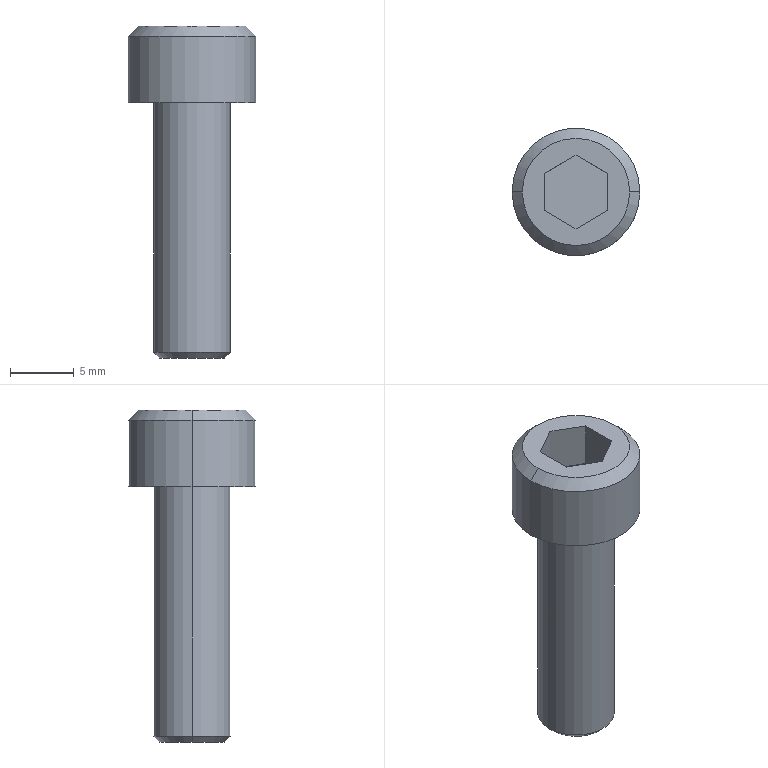Part | Creo | 1 solid | 18 faces | box 10 x 10 x 26 mm | volume 947.453 mm3 | plane 10 | cylinder 4 | cone 4 | commonest cylinder face diameters 6 x2 10 x2
STEP:
#1=CARTESIAN_POINT('',(-109.033,-193.,47.5));
#2=VERTEX_POINT('',#1);
#3=CARTESIAN_POINT('',(-119.033,-193.,47.5));
#4=VERTEX_POINT('',#3);
#5=CARTESIAN_POINT('',(-114.033,-193.,47.5));
#6=DIRECTION('',(0.,0.,-1.));
#7=DIRECTION('',(1.,0.,0.));
#8=AXIS2_PLACEMENT_3D('',#5,#6,#7);
#9=CIRCLE('',#8,5.);
#10=EDGE_CURVE('',#2,#4,#9,.T.);
#11=ORIENTED_EDGE('',*,*,#10,.F.);
#12=CARTESIAN_POINT('',(-114.033,-193.,47.5));
#13=DIRECTION('',(0.,0.,-1.));
#14=DIRECTION('',(-1.,0.,0.));
#15=AXIS2_PLACEMENT_3D('',#12,#13,#14);
#16=CIRCLE('',#15,5.);
#17=EDGE_CURVE('',#4,#2,#16,.T.);
#18=ORIENTED_EDGE('',*,*,#17,.F.);
#19=EDGE_LOOP('',(#11,#18));
#20=FACE_OUTER_BOUND('',#19,.F.);
#21=CARTESIAN_POINT('',(-117.033,-193.,47.5));
#22=VERTEX_POINT('',#21);
#23=CARTESIAN_POINT('',(-111.033,-193.,47.5));
#24=VERTEX_POINT('',#23);
#25=CARTESIAN_POINT('',(-114.033,-193.,47.5));
#26=DIRECTION('',(0.,0.,1.));
#27=DIRECTION('',(-1.,0.,0.));
#28=AXIS2_PLACEMENT_3D('',#25,#26,#27);
#29=CIRCLE('',#28,3.);
#30=EDGE_CURVE('',#22,#24,#29,.T.);
#31=ORIENTED_EDGE('',*,*,#30,.F.);
#32=CARTESIAN_POINT('',(-114.033,-193.,47.5));
#33=DIRECTION('',(0.,0.,1.));
#34=DIRECTION('',(1.,0.,0.));
#35=AXIS2_PLACEMENT_3D('',#32,#33,#34);
#36=CIRCLE('',#35,3.);
#37=EDGE_CURVE('',#24,#22,#36,.T.);
#38=ORIENTED_EDGE('',*,*,#37,.F.);
#39=EDGE_LOOP('',(#31,#38));
#40=FACE_BOUND('',#39,.F.);
#41=CARTESIAN_POINT('',(-114.033,-193.,47.5));
#42=DIRECTION('',(0.,0.,-1.));
#43=DIRECTION('',(-1.,0.,0.));
#44=AXIS2_PLACEMENT_3D('',#41,#42,#43);
#45=PLANE('',#44);
#46=ADVANCED_FACE('',(#20,#40),#45,.T.);
#47=CARTESIAN_POINT('',(-111.033,-193.,27.95));
#48=VERTEX_POINT('',#47);
#49=CARTESIAN_POINT('',(-117.033,-193.,27.95));
#50=VERTEX_POINT('',#49);
#51=CARTESIAN_POINT('',(-114.033,-193.,27.95));
#52=DIRECTION('',(0.,0.,-1.));
#53=DIRECTION('',(1.,0.,0.));
#54=AXIS2_PLACEMENT_3D('',#51,#52,#53);
#55=CIRCLE('',#54,3.);
#56=EDGE_CURVE('',#48,#50,#55,.T.);
#57=ORIENTED_EDGE('',*,*,#56,.T.);
#58=CARTESIAN_POINT('',(-117.033,-193.,47.5));
#59=DIRECTION('',(0.,0.,-1.));
#60=VECTOR('',#59,19.55);
#61=LINE('',#58,#60);
#62=EDGE_CURVE('',#22,#50,#61,.T.);
#63=ORIENTED_EDGE('',*,*,#62,.F.);
#64=ORIENTED_EDGE('',*,*,#30,.T.);
#65=CARTESIAN_POINT('',(-111.033,-193.,47.5));
#66=DIRECTION('',(0.,0.,-1.));
#67=VECTOR('',#66,19.55);
#68=LINE('',#65,#67);
#69=EDGE_CURVE('',#24,#48,#68,.T.);
#70=ORIENTED_EDGE('',*,*,#69,.T.);
#71=EDGE_LOOP('',(#57,#63,#64,#70));
#72=FACE_OUTER_BOUND('',#71,.F.);
#73=CARTESIAN_POINT('',(-114.033,-193.,54.5));
#74=DIRECTION('',(0.,0.,-1.));
#75=DIRECTION('',(-1.,0.,0.));
#76=AXIS2_PLACEMENT_3D('',#73,#74,#75);
#77=CYLINDRICAL_SURFACE('',#76,3.);
#78=ADVANCED_FACE('',(#72),#77,.T.);
#79=CARTESIAN_POINT('',(-111.483,-193.,27.5));
#80=VERTEX_POINT('',#79);
#81=CARTESIAN_POINT('',(-116.583,-193.,27.5));
#82=VERTEX_POINT('',#81);
#83=CARTESIAN_POINT('',(-114.033,-193.,27.5));
#84=DIRECTION('',(0.,0.,-1.));
#85=DIRECTION('',(1.,0.,0.));
#86=AXIS2_PLACEMENT_3D('',#83,#84,#85);
#87=CIRCLE('',#86,2.55);
#88=EDGE_CURVE('',#80,#82,#87,.T.);
#89=ORIENTED_EDGE('',*,*,#88,.T.);
#90=CARTESIAN_POINT('',(-116.583,-193.,27.5));
#91=DIRECTION('',(-0.7071,0.,0.7071));
#92=VECTOR('',#91,0.6364);
#93=LINE('',#90,#92);
#94=EDGE_CURVE('',#82,#50,#93,.T.);
#95=ORIENTED_EDGE('',*,*,#94,.T.);
#96=ORIENTED_EDGE('',*,*,#56,.F.);
#97=CARTESIAN_POINT('',(-111.483,-193.,27.5));
#98=DIRECTION('',(0.7071,0.,0.7071));
#99=VECTOR('',#98,0.6364);
#100=LINE('',#97,#99);
#101=EDGE_CURVE('',#80,#48,#100,.T.);
#102=ORIENTED_EDGE('',*,*,#101,.F.);
#103=EDGE_LOOP('',(#89,#95,#96,#102));
#104=FACE_OUTER_BOUND('',#103,.F.);
#105=CARTESIAN_POINT('',(-114.033,-193.,27.725));
#106=DIRECTION('',(0.,0.,1.));
#107=DIRECTION('',(1.,0.,0.));
#108=AXIS2_PLACEMENT_3D('',#105,#106,#107);
#109=CONICAL_SURFACE('',#108,2.775,45.);
#110=ADVANCED_FACE('',(#104),#109,.T.);
#111=CARTESIAN_POINT('',(-114.033,-193.,27.5));
#112=DIRECTION('',(0.,0.,-1.));
#113=DIRECTION('',(-1.,0.,0.));
#114=AXIS2_PLACEMENT_3D('',#111,#112,#113);
#115=CIRCLE('',#114,2.55);
#116=EDGE_CURVE('',#82,#80,#115,.T.);
#117=ORIENTED_EDGE('',*,*,#116,.F.);
#118=ORIENTED_EDGE('',*,*,#88,.F.);
#119=EDGE_LOOP('',(#117,#118));
#120=FACE_OUTER_BOUND('',#119,.F.);
#121=CARTESIAN_POINT('',(-114.033,-193.,27.5));
#122=DIRECTION('',(0.,0.,-1.));
#123=DIRECTION('',(-1.,0.,0.));
#124=AXIS2_PLACEMENT_3D('',#121,#122,#123);
#125=PLANE('',#124);
#126=ADVANCED_FACE('',(#120),#125,.T.);
#127=ORIENTED_EDGE('',*,*,#116,.T.);
#128=ORIENTED_EDGE('',*,*,#101,.T.);
#129=CARTESIAN_POINT('',(-114.033,-193.,27.95));
#130=DIRECTION('',(0.,0.,-1.));
#131=DIRECTION('',(-1.,0.,0.));
#132=AXIS2_PLACEMENT_3D('',#129,#130,#131);
#133=CIRCLE('',#132,3.);
#134=EDGE_CURVE('',#50,#48,#133,.T.);
#135=ORIENTED_EDGE('',*,*,#134,.F.);
#136=ORIENTED_EDGE('',*,*,#94,.F.);
#137=EDGE_LOOP('',(#127,#128,#135,#136));
#138=FACE_OUTER_BOUND('',#137,.F.);
#139=CARTESIAN_POINT('',(-114.033,-193.,27.725));
#140=DIRECTION('',(0.,0.,1.));
#141=DIRECTION('',(1.,0.,0.));
#142=AXIS2_PLACEMENT_3D('',#139,#140,#141);
#143=CONICAL_SURFACE('',#142,2.775,45.);
#144=ADVANCED_FACE('',(#138),#143,.T.);
#145=ORIENTED_EDGE('',*,*,#134,.T.);
#146=ORIENTED_EDGE('',*,*,#69,.F.);
#147=ORIENTED_EDGE('',*,*,#37,.T.);
#148=ORIENTED_EDGE('',*,*,#62,.T.);
#149=EDGE_LOOP('',(#145,#146,#147,#148));
#150=FACE_OUTER_BOUND('',#149,.F.);
#151=CARTESIAN_POINT('',(-114.033,-193.,54.5));
#152=DIRECTION('',(0.,0.,-1.));
#153=DIRECTION('',(-1.,0.,0.));
#154=AXIS2_PLACEMENT_3D('',#151,#152,#153);
#155=CYLINDRICAL_SURFACE('',#154,3.);
#156=ADVANCED_FACE('',(#150),#155,.T.);
#157=CARTESIAN_POINT('',(-119.033,-193.,52.7));
#158=VERTEX_POINT('',#157);
#159=CARTESIAN_POINT('',(-109.033,-193.,52.7));
#160=VERTEX_POINT('',#159);
#161=CARTESIAN_POINT('',(-114.033,-193.,52.7));
#162=DIRECTION('',(0.,0.,1.));
#163=DIRECTION('',(-1.,0.,0.));
#164=AXIS2_PLACEMENT_3D('',#161,#162,#163);
#165=CIRCLE('',#164,5.);
#166=EDGE_CURVE('',#158,#160,#165,.T.);
#167=ORIENTED_EDGE('',*,*,#166,.T.);
#168=CARTESIAN_POINT('',(-109.033,-193.,52.7));
#169=DIRECTION('',(0.,0.,-1.));
#170=VECTOR('',#169,5.2);
#171=LINE('',#168,#170);
#172=EDGE_CURVE('',#160,#2,#171,.T.);
#173=ORIENTED_EDGE('',*,*,#172,.T.);
#174=ORIENTED_EDGE('',*,*,#10,.T.);
#175=CARTESIAN_POINT('',(-119.033,-193.,52.7));
#176=DIRECTION('',(0.,0.,-1.));
#177=VECTOR('',#176,5.2);
#178=LINE('',#175,#177);
#179=EDGE_CURVE('',#158,#4,#178,.T.);
#180=ORIENTED_EDGE('',*,*,#179,.F.);
#181=EDGE_LOOP('',(#167,#173,#174,#180));
#182=FACE_OUTER_BOUND('',#181,.F.);
#183=CARTESIAN_POINT('',(-114.033,-193.,54.5));
#184=DIRECTION('',(0.,0.,-1.));
#185=DIRECTION('',(-1.,0.,0.));
#186=AXIS2_PLACEMENT_3D('',#183,#184,#185);
#187=CYLINDRICAL_SURFACE('',#186,5.);
#188=ADVANCED_FACE('',(#182),#187,.T.);
#189=CARTESIAN_POINT('',(-118.233,-193.,53.5));
#190=VERTEX_POINT('',#189);
#191=CARTESIAN_POINT('',(-109.833,-193.,53.5));
#192=VERTEX_POINT('',#191);
#193=CARTESIAN_POINT('',(-114.033,-193.,53.5));
#194=DIRECTION('',(0.,0.,1.));
#195=DIRECTION('',(-1.,0.,0.));
#196=AXIS2_PLACEMENT_3D('',#193,#194,#195);
#197=CIRCLE('',#196,4.2);
#198=EDGE_CURVE('',#190,#192,#197,.T.);
#199=ORIENTED_EDGE('',*,*,#198,.T.);
#200=CARTESIAN_POINT('',(-109.833,-193.,53.5));
#201=DIRECTION('',(0.7071,0.,-0.7071));
#202=VECTOR('',#201,1.131);
#203=LINE('',#200,#202);
#204=EDGE_CURVE('',#192,#160,#203,.T.);
#205=ORIENTED_EDGE('',*,*,#204,.T.);
#206=ORIENTED_EDGE('',*,*,#166,.F.);
#207=CARTESIAN_POINT('',(-118.233,-193.,53.5));
#208=DIRECTION('',(-0.7071,0.,-0.7071));
#209=VECTOR('',#208,1.131);
#210=LINE('',#207,#209);
#211=EDGE_CURVE('',#190,#158,#210,.T.);
#212=ORIENTED_EDGE('',*,*,#211,.F.);
#213=EDGE_LOOP('',(#199,#205,#206,#212));
#214=FACE_OUTER_BOUND('',#213,.F.);
#215=CARTESIAN_POINT('',(-114.033,-193.,53.1));
#216=DIRECTION('',(0.,0.,-1.));
#217=DIRECTION('',(-1.,0.,0.));
#218=AXIS2_PLACEMENT_3D('',#215,#216,#217);
#219=CONICAL_SURFACE('',#218,4.6,45.);
#220=ADVANCED_FACE('',(#214),#219,.T.);
#221=ORIENTED_EDGE('',*,*,#198,.F.);
#222=CARTESIAN_POINT('',(-114.033,-193.,53.5));
#223=DIRECTION('',(0.,0.,1.));
#224=DIRECTION('',(1.,0.,0.));
#225=AXIS2_PLACEMENT_3D('',#222,#223,#224);
#226=CIRCLE('',#225,4.2);
#227=EDGE_CURVE('',#192,#190,#226,.T.);
#228=ORIENTED_EDGE('',*,*,#227,.F.);
#229=EDGE_LOOP('',(#221,#228));
#230=FACE_OUTER_BOUND('',#229,.F.);
#231=CARTESIAN_POINT('',(-111.533,-194.443,53.5));
#232=VERTEX_POINT('',#231);
#233=CARTESIAN_POINT('',(-114.033,-195.887,53.5));
#234=VERTEX_POINT('',#233);
#235=CARTESIAN_POINT('',(-111.533,-194.443,53.5));
#236=DIRECTION('',(-0.866,-0.5,0.));
#237=VECTOR('',#236,2.887);
#238=LINE('',#235,#237);
#239=EDGE_CURVE('',#232,#234,#238,.T.);
#240=ORIENTED_EDGE('',*,*,#239,.F.);
#241=CARTESIAN_POINT('',(-111.533,-191.557,53.5));
#242=VERTEX_POINT('',#241);
#243=CARTESIAN_POINT('',(-111.533,-191.557,53.5));
#244=DIRECTION('',(0.,-1.,0.));
#245=VECTOR('',#244,2.887);
#246=LINE('',#243,#245);
#247=EDGE_CURVE('',#242,#232,#246,.T.);
#248=ORIENTED_EDGE('',*,*,#247,.F.);
#249=CARTESIAN_POINT('',(-114.033,-190.113,53.5));
#250=VERTEX_POINT('',#249);
#251=CARTESIAN_POINT('',(-114.033,-190.113,53.5));
#252=DIRECTION('',(0.866,-0.5,0.));
#253=VECTOR('',#252,2.887);
#254=LINE('',#251,#253);
#255=EDGE_CURVE('',#250,#242,#254,.T.);
#256=ORIENTED_EDGE('',*,*,#255,.F.);
#257=CARTESIAN_POINT('',(-116.533,-191.557,53.5));
#258=VERTEX_POINT('',#257);
#259=CARTESIAN_POINT('',(-116.533,-191.557,53.5));
#260=DIRECTION('',(0.866,0.5,0.));
#261=VECTOR('',#260,2.887);
#262=LINE('',#259,#261);
#263=EDGE_CURVE('',#258,#250,#262,.T.);
#264=ORIENTED_EDGE('',*,*,#263,.F.);
#265=CARTESIAN_POINT('',(-116.533,-194.443,53.5));
#266=VERTEX_POINT('',#265);
#267=CARTESIAN_POINT('',(-116.533,-194.443,53.5));
#268=DIRECTION('',(0.,1.,0.));
#269=VECTOR('',#268,2.887);
#270=LINE('',#267,#269);
#271=EDGE_CURVE('',#266,#258,#270,.T.);
#272=ORIENTED_EDGE('',*,*,#271,.F.);
#273=CARTESIAN_POINT('',(-114.033,-195.887,53.5));
#274=DIRECTION('',(-0.866,0.5,0.));
#275=VECTOR('',#274,2.887);
#276=LINE('',#273,#275);
#277=EDGE_CURVE('',#234,#266,#276,.T.);
#278=ORIENTED_EDGE('',*,*,#277,.F.);
#279=EDGE_LOOP('',(#240,#248,#256,#264,#272,#278));
#280=FACE_BOUND('',#279,.F.);
#281=CARTESIAN_POINT('',(-114.033,-193.,53.5));
#282=DIRECTION('',(0.,0.,-1.));
#283=DIRECTION('',(-1.,0.,0.));
#284=AXIS2_PLACEMENT_3D('',#281,#282,#283);
#285=PLANE('',#284);
#286=ADVANCED_FACE('',(#230,#280),#285,.F.);
#287=ORIENTED_EDGE('',*,*,#227,.T.);
#288=ORIENTED_EDGE('',*,*,#211,.T.);
#289=CARTESIAN_POINT('',(-114.033,-193.,52.7));
#290=DIRECTION('',(0.,0.,1.));
#291=DIRECTION('',(1.,0.,0.));
#292=AXIS2_PLACEMENT_3D('',#289,#290,#291);
#293=CIRCLE('',#292,5.);
#294=EDGE_CURVE('',#160,#158,#293,.T.);
#295=ORIENTED_EDGE('',*,*,#294,.F.);
#296=ORIENTED_EDGE('',*,*,#204,.F.);
#297=EDGE_LOOP('',(#287,#288,#295,#296));
#298=FACE_OUTER_BOUND('',#297,.F.);
#299=CARTESIAN_POINT('',(-114.033,-193.,53.1));
#300=DIRECTION('',(0.,0.,-1.));
#301=DIRECTION('',(-1.,0.,0.));
#302=AXIS2_PLACEMENT_3D('',#299,#300,#301);
#303=CONICAL_SURFACE('',#302,4.6,45.);
#304=ADVANCED_FACE('',(#298),#303,.T.);
#305=ORIENTED_EDGE('',*,*,#294,.T.);
#306=ORIENTED_EDGE('',*,*,#179,.T.);
#307=ORIENTED_EDGE('',*,*,#17,.T.);
#308=ORIENTED_EDGE('',*,*,#172,.F.);
#309=EDGE_LOOP('',(#305,#306,#307,#308));
#310=FACE_OUTER_BOUND('',#309,.F.);
#311=CARTESIAN_POINT('',(-114.033,-193.,54.5));
#312=DIRECTION('',(0.,0.,-1.));
#313=DIRECTION('',(-1.,0.,0.));
#314=AXIS2_PLACEMENT_3D('',#311,#312,#313);
#315=CYLINDRICAL_SURFACE('',#314,5.);
#316=ADVANCED_FACE('',(#310),#315,.T.);
#317=ORIENTED_EDGE('',*,*,#239,.T.);
#318=CARTESIAN_POINT('',(-114.033,-195.887,49.9));
#319=VERTEX_POINT('',#318);
#320=CARTESIAN_POINT('',(-114.033,-195.887,53.5));
#321=DIRECTION('',(0.,0.,-1.));
#322=VECTOR('',#321,3.6);
#323=LINE('',#320,#322);
#324=EDGE_CURVE('',#234,#319,#323,.T.);
#325=ORIENTED_EDGE('',*,*,#324,.T.);
#326=CARTESIAN_POINT('',(-111.533,-194.443,49.9));
#327=VERTEX_POINT('',#326);
#328=CARTESIAN_POINT('',(-114.033,-195.887,49.9));
#329=DIRECTION('',(0.866,0.5,0.));
#330=VECTOR('',#329,2.887);
#331=LINE('',#328,#330);
#332=EDGE_CURVE('',#319,#327,#331,.T.);
#333=ORIENTED_EDGE('',*,*,#332,.T.);
#334=CARTESIAN_POINT('',(-111.533,-194.443,53.5));
#335=DIRECTION('',(0.,0.,-1.));
#336=VECTOR('',#335,3.6);
#337=LINE('',#334,#336);
#338=EDGE_CURVE('',#232,#327,#337,.T.);
#339=ORIENTED_EDGE('',*,*,#338,.F.);
#340=EDGE_LOOP('',(#317,#325,#333,#339));
#341=FACE_OUTER_BOUND('',#340,.F.);
#342=CARTESIAN_POINT('',(-114.033,-195.887,49.9));
#343=DIRECTION('',(0.5,-0.866,0.));
#344=DIRECTION('',(0.866,0.5,0.));
#345=AXIS2_PLACEMENT_3D('',#342,#343,#344);
#346=PLANE('',#345);
#347=ADVANCED_FACE('',(#341),#346,.F.);
#348=ORIENTED_EDGE('',*,*,#277,.T.);
#349=CARTESIAN_POINT('',(-116.533,-194.443,49.9));
#350=VERTEX_POINT('',#349);
#351=CARTESIAN_POINT('',(-116.533,-194.443,53.5));
#352=DIRECTION('',(0.,0.,-1.));
#353=VECTOR('',#352,3.6);
#354=LINE('',#351,#353);
#355=EDGE_CURVE('',#266,#350,#354,.T.);
#356=ORIENTED_EDGE('',*,*,#355,.T.);
#357=CARTESIAN_POINT('',(-116.533,-194.443,49.9));
#358=DIRECTION('',(0.866,-0.5,0.));
#359=VECTOR('',#358,2.887);
#360=LINE('',#357,#359);
#361=EDGE_CURVE('',#350,#319,#360,.T.);
#362=ORIENTED_EDGE('',*,*,#361,.T.);
#363=ORIENTED_EDGE('',*,*,#324,.F.);
#364=EDGE_LOOP('',(#348,#356,#362,#363));
#365=FACE_OUTER_BOUND('',#364,.F.);
#366=CARTESIAN_POINT('',(-116.533,-194.443,49.9));
#367=DIRECTION('',(-0.5,-0.866,0.));
#368=DIRECTION('',(0.866,-0.5,0.));
#369=AXIS2_PLACEMENT_3D('',#366,#367,#368);
#370=PLANE('',#369);
#371=ADVANCED_FACE('',(#365),#370,.F.);
#372=ORIENTED_EDGE('',*,*,#271,.T.);
#373=CARTESIAN_POINT('',(-116.533,-191.557,49.9));
#374=VERTEX_POINT('',#373);
#375=CARTESIAN_POINT('',(-116.533,-191.557,53.5));
#376=DIRECTION('',(0.,0.,-1.));
#377=VECTOR('',#376,3.6);
#378=LINE('',#375,#377);
#379=EDGE_CURVE('',#258,#374,#378,.T.);
#380=ORIENTED_EDGE('',*,*,#379,.T.);
#381=CARTESIAN_POINT('',(-116.533,-194.443,49.9));
#382=DIRECTION('',(0.,1.,0.));
#383=VECTOR('',#382,2.887);
#384=LINE('',#381,#383);
#385=EDGE_CURVE('',#350,#374,#384,.T.);
#386=ORIENTED_EDGE('',*,*,#385,.F.);
#387=ORIENTED_EDGE('',*,*,#355,.F.);
#388=EDGE_LOOP('',(#372,#380,#386,#387));
#389=FACE_OUTER_BOUND('',#388,.F.);
#390=CARTESIAN_POINT('',(-116.533,-191.557,49.9));
#391=DIRECTION('',(-1.,0.,0.));
#392=DIRECTION('',(0.,0.,1.));
#393=AXIS2_PLACEMENT_3D('',#390,#391,#392);
#394=PLANE('',#393);
#395=ADVANCED_FACE('',(#389),#394,.F.);
#396=ORIENTED_EDGE('',*,*,#263,.T.);
#397=CARTESIAN_POINT('',(-114.033,-190.113,49.9));
#398=VERTEX_POINT('',#397);
#399=CARTESIAN_POINT('',(-114.033,-190.113,53.5));
#400=DIRECTION('',(0.,0.,-1.));
#401=VECTOR('',#400,3.6);
#402=LINE('',#399,#401);
#403=EDGE_CURVE('',#250,#398,#402,.T.);
#404=ORIENTED_EDGE('',*,*,#403,.T.);
#405=CARTESIAN_POINT('',(-114.033,-190.113,49.9));
#406=DIRECTION('',(-0.866,-0.5,0.));
#407=VECTOR('',#406,2.887);
#408=LINE('',#405,#407);
#409=EDGE_CURVE('',#398,#374,#408,.T.);
#410=ORIENTED_EDGE('',*,*,#409,.T.);
#411=ORIENTED_EDGE('',*,*,#379,.F.);
#412=EDGE_LOOP('',(#396,#404,#410,#411));
#413=FACE_OUTER_BOUND('',#412,.F.);
#414=CARTESIAN_POINT('',(-114.033,-190.113,49.9));
#415=DIRECTION('',(-0.5,0.866,0.));
#416=DIRECTION('',(-0.866,-0.5,0.));
#417=AXIS2_PLACEMENT_3D('',#414,#415,#416);
#418=PLANE('',#417);
#419=ADVANCED_FACE('',(#413),#418,.F.);
#420=ORIENTED_EDGE('',*,*,#255,.T.);
#421=CARTESIAN_POINT('',(-111.533,-191.557,49.9));
#422=VERTEX_POINT('',#421);
#423=CARTESIAN_POINT('',(-111.533,-191.557,53.5));
#424=DIRECTION('',(0.,0.,-1.));
#425=VECTOR('',#424,3.6);
#426=LINE('',#423,#425);
#427=EDGE_CURVE('',#242,#422,#426,.T.);
#428=ORIENTED_EDGE('',*,*,#427,.T.);
#429=CARTESIAN_POINT('',(-111.533,-191.557,49.9));
#430=DIRECTION('',(-0.866,0.5,0.));
#431=VECTOR('',#430,2.887);
#432=LINE('',#429,#431);
#433=EDGE_CURVE('',#422,#398,#432,.T.);
#434=ORIENTED_EDGE('',*,*,#433,.T.);
#435=ORIENTED_EDGE('',*,*,#403,.F.);
#436=EDGE_LOOP('',(#420,#428,#434,#435));
#437=FACE_OUTER_BOUND('',#436,.F.);
#438=CARTESIAN_POINT('',(-111.533,-191.557,49.9));
#439=DIRECTION('',(0.5,0.866,0.));
#440=DIRECTION('',(-0.866,0.5,0.));
#441=AXIS2_PLACEMENT_3D('',#438,#439,#440);
#442=PLANE('',#441);
#443=ADVANCED_FACE('',(#437),#442,.F.);
#444=ORIENTED_EDGE('',*,*,#247,.T.);
#445=ORIENTED_EDGE('',*,*,#338,.T.);
#446=CARTESIAN_POINT('',(-111.533,-191.557,49.9));
#447=DIRECTION('',(0.,-1.,0.));
#448=VECTOR('',#447,2.887);
#449=LINE('',#446,#448);
#450=EDGE_CURVE('',#422,#327,#449,.T.);
#451=ORIENTED_EDGE('',*,*,#450,.F.);
#452=ORIENTED_EDGE('',*,*,#427,.F.);
#453=EDGE_LOOP('',(#444,#445,#451,#452));
#454=FACE_OUTER_BOUND('',#453,.F.);
#455=CARTESIAN_POINT('',(-111.533,-194.443,49.9));
#456=DIRECTION('',(1.,0.,0.));
#457=DIRECTION('',(0.,0.,-1.));
#458=AXIS2_PLACEMENT_3D('',#455,#456,#457);
#459=PLANE('',#458);
#460=ADVANCED_FACE('',(#454),#459,.F.);
#461=ORIENTED_EDGE('',*,*,#361,.F.);
#462=ORIENTED_EDGE('',*,*,#385,.T.);
#463=ORIENTED_EDGE('',*,*,#409,.F.);
#464=ORIENTED_EDGE('',*,*,#433,.F.);
#465=ORIENTED_EDGE('',*,*,#450,.T.);
#466=ORIENTED_EDGE('',*,*,#332,.F.);
#467=EDGE_LOOP('',(#461,#462,#463,#464,#465,#466));
#468=FACE_OUTER_BOUND('',#467,.F.);
#469=CARTESIAN_POINT('',(-111.533,-197.33,49.9));
#470=DIRECTION('',(0.,0.,1.));
#471=DIRECTION('',(0.,-1.,0.));
#472=AXIS2_PLACEMENT_3D('',#469,#470,#471);
#473=PLANE('',#472);
#474=ADVANCED_FACE('',(#468),#473,.T.);
#475=CLOSED_SHELL('',(#46,#78,#110,#126,#144,#156,#188,#220,#286,#304,#316,#347,#371,#395,#419,#443,#460,#474));
#476=MANIFOLD_SOLID_BREP('',#475);
#477=(LENGTH_UNIT()NAMED_UNIT(*)SI_UNIT(.MILLI.,.METRE.));
#478=UNCERTAINTY_MEASURE_WITH_UNIT(LENGTH_MEASURE(0.00296),#477,'','');
#479=(NAMED_UNIT(*)PLANE_ANGLE_UNIT()SI_UNIT($,.RADIAN.));
#480=PLANE_ANGLE_MEASURE_WITH_UNIT(PLANE_ANGLE_MEASURE(0.01745),#479);
#481=(CONVERSION_BASED_UNIT('DEGREE',#480)NAMED_UNIT(*)PLANE_ANGLE_UNIT());
#482=(NAMED_UNIT(*)SI_UNIT($,.STERADIAN.)SOLID_ANGLE_UNIT());
#483=(GEOMETRIC_REPRESENTATION_CONTEXT(3)GLOBAL_UNCERTAINTY_ASSIGNED_CONTEXT((#478))GLOBAL_UNIT_ASSIGNED_CONTEXT((#477,#481,#482))REPRESENTATION_CONTEXT('',''));
#484=ADVANCED_BREP_SHAPE_REPRESENTATION('',(#476),#483);